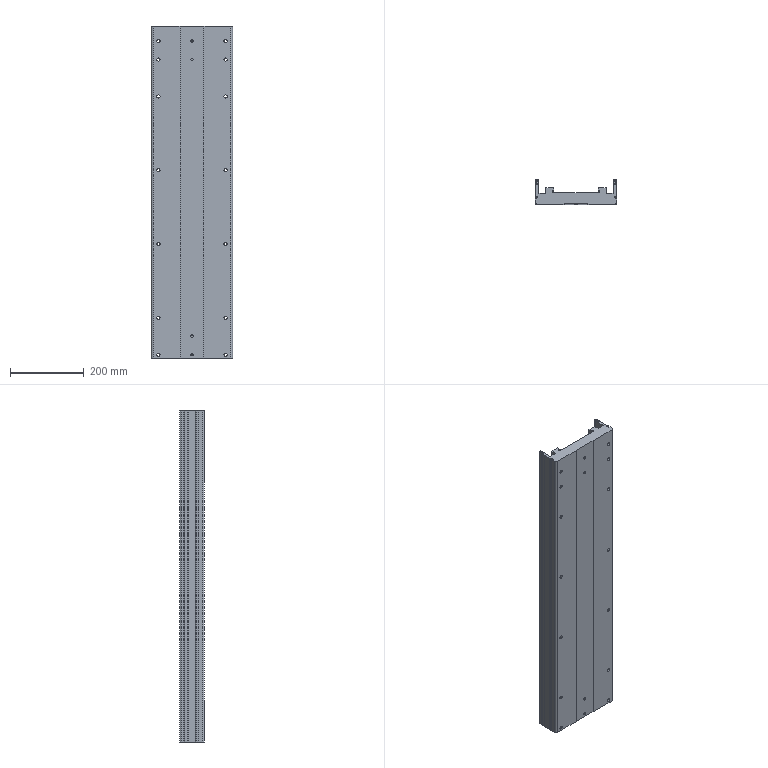Part | SolidWorks | features HoleWzd 3, ICE 3, Extrusion 1, Fillet 1, LPattern 1 | 1 solid | 212 faces | box 220 x 67.5 x 900 mm | volume 6810369 mm3 | plane 114 | cylinder 98 | commonest cylinder face diameters 8.6 x28 15 x28 0.4 x12 6 x10 4.2 x9 10 x4